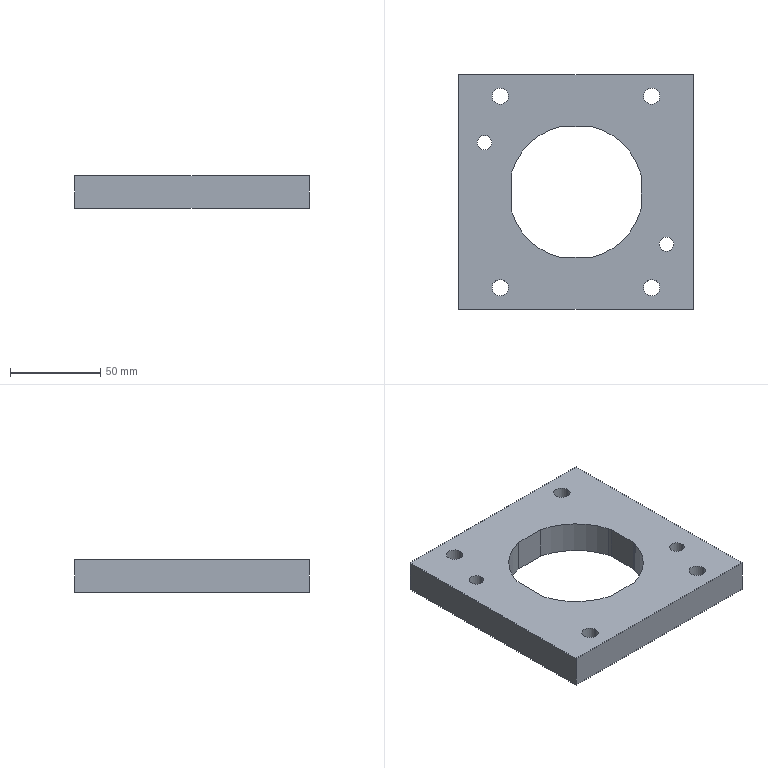Part | SolidWorks | features BaseBody 1 | 1 solid | 30 faces | box 130 x 130 x 18 mm | volume 220294 mm3 | cylinder 18 | plane 12 | commonest cylinder face diameters 9.007 x8 8 x4 74.52 x4 74.5 x2
STEP:
#1=CARTESIAN_POINT('',(-123.497,-77.99,46.3));
#2=VERTEX_POINT('',#1);
#3=CARTESIAN_POINT('',(-132.504,-77.99,46.3));
#4=VERTEX_POINT('',#3);
#5=CARTESIAN_POINT('',(-128.,-77.99,46.3));
#6=DIRECTION('',(0.,0.,-1.));
#7=DIRECTION('',(0.7071,-0.7071,0.));
#8=AXIS2_PLACEMENT_3D('',#5,#6,#7);
#9=CIRCLE('',#8,4.503);
#10=EDGE_CURVE('',#2,#4,#9,.T.);
#11=ORIENTED_EDGE('',*,*,#10,.T.);
#12=CARTESIAN_POINT('',(-132.504,-77.99,64.3));
#13=VERTEX_POINT('',#12);
#14=CARTESIAN_POINT('',(-132.504,-77.99,46.3));
#15=DIRECTION('',(0.,0.,1.));
#16=VECTOR('',#15,1000.);
#17=LINE('',#14,#16);
#18=EDGE_CURVE('',#4,#13,#17,.T.);
#19=ORIENTED_EDGE('',*,*,#18,.T.);
#20=CARTESIAN_POINT('',(-123.497,-77.99,64.3));
#21=VERTEX_POINT('',#20);
#22=CARTESIAN_POINT('',(-128.,-77.99,64.3));
#23=DIRECTION('',(0.,0.,-1.));
#24=DIRECTION('',(0.7071,-0.7071,0.));
#25=AXIS2_PLACEMENT_3D('',#22,#23,#24);
#26=CIRCLE('',#25,4.503);
#27=EDGE_CURVE('',#21,#13,#26,.T.);
#28=ORIENTED_EDGE('',*,*,#27,.F.);
#29=CARTESIAN_POINT('',(-123.497,-77.99,46.3));
#30=DIRECTION('',(0.,0.,1.));
#31=VECTOR('',#30,1000.);
#32=LINE('',#29,#31);
#33=EDGE_CURVE('',#2,#21,#32,.T.);
#34=ORIENTED_EDGE('',*,*,#33,.F.);
#35=EDGE_LOOP('',(#11,#19,#28,#34));
#36=FACE_OUTER_BOUND('',#35,.T.);
#37=CARTESIAN_POINT('',(-128.,-77.99,46.3));
#38=DIRECTION('',(0.,0.,1.));
#39=DIRECTION('',(1.,0.,0.));
#40=AXIS2_PLACEMENT_3D('',#37,#38,#39);
#41=CYLINDRICAL_SURFACE('',#40,4.503);
#42=ADVANCED_FACE('',(#36),#41,.F.);
#43=CARTESIAN_POINT('',(-48.503,27.99,46.3));
#44=VERTEX_POINT('',#43);
#45=CARTESIAN_POINT('',(-39.496,27.99,46.3));
#46=VERTEX_POINT('',#45);
#47=CARTESIAN_POINT('',(-44.,27.99,46.3));
#48=DIRECTION('',(0.,0.,-1.));
#49=DIRECTION('',(-0.7071,0.7071,0.));
#50=AXIS2_PLACEMENT_3D('',#47,#48,#49);
#51=CIRCLE('',#50,4.503);
#52=EDGE_CURVE('',#44,#46,#51,.T.);
#53=ORIENTED_EDGE('',*,*,#52,.T.);
#54=CARTESIAN_POINT('',(-39.496,27.99,64.3));
#55=VERTEX_POINT('',#54);
#56=CARTESIAN_POINT('',(-39.496,27.99,46.3));
#57=DIRECTION('',(0.,0.,1.));
#58=VECTOR('',#57,1000.);
#59=LINE('',#56,#58);
#60=EDGE_CURVE('',#46,#55,#59,.T.);
#61=ORIENTED_EDGE('',*,*,#60,.T.);
#62=CARTESIAN_POINT('',(-48.503,27.99,64.3));
#63=VERTEX_POINT('',#62);
#64=CARTESIAN_POINT('',(-44.,27.99,64.3));
#65=DIRECTION('',(0.,0.,-1.));
#66=DIRECTION('',(-0.7071,0.7071,0.));
#67=AXIS2_PLACEMENT_3D('',#64,#65,#66);
#68=CIRCLE('',#67,4.503);
#69=EDGE_CURVE('',#63,#55,#68,.T.);
#70=ORIENTED_EDGE('',*,*,#69,.F.);
#71=CARTESIAN_POINT('',(-48.503,27.99,46.3));
#72=DIRECTION('',(0.,0.,1.));
#73=VECTOR('',#72,1000.);
#74=LINE('',#71,#73);
#75=EDGE_CURVE('',#44,#63,#74,.T.);
#76=ORIENTED_EDGE('',*,*,#75,.F.);
#77=EDGE_LOOP('',(#53,#61,#70,#76));
#78=FACE_OUTER_BOUND('',#77,.T.);
#79=CARTESIAN_POINT('',(-44.,27.99,46.3));
#80=DIRECTION('',(0.,0.,1.));
#81=DIRECTION('',(-1.,0.,0.));
#82=AXIS2_PLACEMENT_3D('',#79,#80,#81);
#83=CYLINDRICAL_SURFACE('',#82,4.504);
#84=ADVANCED_FACE('',(#78),#83,.F.);
#85=CARTESIAN_POINT('',(-140.678,2.312,46.3));
#86=VERTEX_POINT('',#85);
#87=CARTESIAN_POINT('',(-132.678,2.312,46.3));
#88=VERTEX_POINT('',#87);
#89=CARTESIAN_POINT('',(-136.678,2.312,46.3));
#90=DIRECTION('',(0.,0.,1.));
#91=DIRECTION('',(0.7071,0.7071,0.));
#92=AXIS2_PLACEMENT_3D('',#89,#90,#91);
#93=CIRCLE('',#92,4.);
#94=EDGE_CURVE('',#86,#88,#93,.T.);
#95=ORIENTED_EDGE('',*,*,#94,.F.);
#96=CARTESIAN_POINT('',(-140.678,2.312,64.3));
#97=VERTEX_POINT('',#96);
#98=CARTESIAN_POINT('',(-140.678,2.312,46.3));
#99=DIRECTION('',(0.,0.,1.));
#100=VECTOR('',#99,1000.);
#101=LINE('',#98,#100);
#102=EDGE_CURVE('',#86,#97,#101,.T.);
#103=ORIENTED_EDGE('',*,*,#102,.T.);
#104=CARTESIAN_POINT('',(-132.678,2.312,64.3));
#105=VERTEX_POINT('',#104);
#106=CARTESIAN_POINT('',(-136.678,2.312,64.3));
#107=DIRECTION('',(0.,0.,1.));
#108=DIRECTION('',(0.7071,0.7071,0.));
#109=AXIS2_PLACEMENT_3D('',#106,#107,#108);
#110=CIRCLE('',#109,4.);
#111=EDGE_CURVE('',#97,#105,#110,.T.);
#112=ORIENTED_EDGE('',*,*,#111,.T.);
#113=CARTESIAN_POINT('',(-132.678,2.312,46.3));
#114=DIRECTION('',(0.,0.,1.));
#115=VECTOR('',#114,1000.);
#116=LINE('',#113,#115);
#117=EDGE_CURVE('',#88,#105,#116,.T.);
#118=ORIENTED_EDGE('',*,*,#117,.F.);
#119=EDGE_LOOP('',(#95,#103,#112,#118));
#120=FACE_OUTER_BOUND('',#119,.T.);
#121=CARTESIAN_POINT('',(-136.678,2.312,46.3));
#122=DIRECTION('',(0.,0.,1.));
#123=DIRECTION('',(1.,0.,0.));
#124=AXIS2_PLACEMENT_3D('',#121,#122,#123);
#125=CYLINDRICAL_SURFACE('',#124,4.);
#126=ADVANCED_FACE('',(#120),#125,.F.);
#127=CARTESIAN_POINT('',(-39.858,-53.934,46.3));
#128=VERTEX_POINT('',#127);
#129=CARTESIAN_POINT('',(-31.858,-53.934,46.3));
#130=VERTEX_POINT('',#129);
#131=CARTESIAN_POINT('',(-35.858,-53.934,46.3));
#132=DIRECTION('',(0.,0.,1.));
#133=DIRECTION('',(0.7071,0.7071,0.));
#134=AXIS2_PLACEMENT_3D('',#131,#132,#133);
#135=CIRCLE('',#134,4.);
#136=EDGE_CURVE('',#128,#130,#135,.T.);
#137=ORIENTED_EDGE('',*,*,#136,.F.);
#138=CARTESIAN_POINT('',(-39.858,-53.934,64.3));
#139=VERTEX_POINT('',#138);
#140=CARTESIAN_POINT('',(-39.858,-53.934,46.3));
#141=DIRECTION('',(0.,0.,1.));
#142=VECTOR('',#141,1000.);
#143=LINE('',#140,#142);
#144=EDGE_CURVE('',#128,#139,#143,.T.);
#145=ORIENTED_EDGE('',*,*,#144,.T.);
#146=CARTESIAN_POINT('',(-31.858,-53.934,64.3));
#147=VERTEX_POINT('',#146);
#148=CARTESIAN_POINT('',(-35.858,-53.934,64.3));
#149=DIRECTION('',(0.,0.,1.));
#150=DIRECTION('',(0.7071,0.7071,0.));
#151=AXIS2_PLACEMENT_3D('',#148,#149,#150);
#152=CIRCLE('',#151,4.);
#153=EDGE_CURVE('',#139,#147,#152,.T.);
#154=ORIENTED_EDGE('',*,*,#153,.T.);
#155=CARTESIAN_POINT('',(-31.858,-53.934,46.3));
#156=DIRECTION('',(0.,0.,1.));
#157=VECTOR('',#156,1000.);
#158=LINE('',#155,#157);
#159=EDGE_CURVE('',#130,#147,#158,.T.);
#160=ORIENTED_EDGE('',*,*,#159,.F.);
#161=EDGE_LOOP('',(#137,#145,#154,#160));
#162=FACE_OUTER_BOUND('',#161,.T.);
#163=CARTESIAN_POINT('',(-35.858,-53.934,46.3));
#164=DIRECTION('',(0.,0.,1.));
#165=DIRECTION('',(1.,0.,0.));
#166=AXIS2_PLACEMENT_3D('',#163,#164,#165);
#167=CYLINDRICAL_SURFACE('',#166,4.);
#168=ADVANCED_FACE('',(#162),#167,.F.);
#169=CARTESIAN_POINT('',(-39.496,-77.99,46.3));
#170=VERTEX_POINT('',#169);
#171=CARTESIAN_POINT('',(-48.503,-77.99,46.3));
#172=VERTEX_POINT('',#171);
#173=CARTESIAN_POINT('',(-44.,-77.99,46.3));
#174=DIRECTION('',(0.,0.,1.));
#175=DIRECTION('',(-0.7071,-0.7071,0.));
#176=AXIS2_PLACEMENT_3D('',#173,#174,#175);
#177=CIRCLE('',#176,4.503);
#178=EDGE_CURVE('',#170,#172,#177,.T.);
#179=ORIENTED_EDGE('',*,*,#178,.F.);
#180=CARTESIAN_POINT('',(-39.496,-77.99,64.3));
#181=VERTEX_POINT('',#180);
#182=CARTESIAN_POINT('',(-39.496,-77.99,46.3));
#183=DIRECTION('',(0.,0.,1.));
#184=VECTOR('',#183,1000.);
#185=LINE('',#182,#184);
#186=EDGE_CURVE('',#170,#181,#185,.T.);
#187=ORIENTED_EDGE('',*,*,#186,.T.);
#188=CARTESIAN_POINT('',(-48.503,-77.99,64.3));
#189=VERTEX_POINT('',#188);
#190=CARTESIAN_POINT('',(-44.,-77.99,64.3));
#191=DIRECTION('',(0.,0.,1.));
#192=DIRECTION('',(-0.7071,-0.7071,0.));
#193=AXIS2_PLACEMENT_3D('',#190,#191,#192);
#194=CIRCLE('',#193,4.503);
#195=EDGE_CURVE('',#181,#189,#194,.T.);
#196=ORIENTED_EDGE('',*,*,#195,.T.);
#197=CARTESIAN_POINT('',(-48.503,-77.99,46.3));
#198=DIRECTION('',(0.,0.,1.));
#199=VECTOR('',#198,1000.);
#200=LINE('',#197,#199);
#201=EDGE_CURVE('',#172,#189,#200,.T.);
#202=ORIENTED_EDGE('',*,*,#201,.F.);
#203=EDGE_LOOP('',(#179,#187,#196,#202));
#204=FACE_OUTER_BOUND('',#203,.T.);
#205=CARTESIAN_POINT('',(-44.,-77.99,46.3));
#206=DIRECTION('',(0.,0.,1.));
#207=DIRECTION('',(-1.,0.,0.));
#208=AXIS2_PLACEMENT_3D('',#205,#206,#207);
#209=CYLINDRICAL_SURFACE('',#208,4.504);
#210=ADVANCED_FACE('',(#204),#209,.F.);
#211=CARTESIAN_POINT('',(-132.504,27.99,46.3));
#212=VERTEX_POINT('',#211);
#213=CARTESIAN_POINT('',(-123.497,27.99,46.3));
#214=VERTEX_POINT('',#213);
#215=CARTESIAN_POINT('',(-128.,27.99,46.3));
#216=DIRECTION('',(0.,0.,1.));
#217=DIRECTION('',(0.7071,0.7071,0.));
#218=AXIS2_PLACEMENT_3D('',#215,#216,#217);
#219=CIRCLE('',#218,4.504);
#220=EDGE_CURVE('',#212,#214,#219,.T.);
#221=ORIENTED_EDGE('',*,*,#220,.F.);
#222=CARTESIAN_POINT('',(-132.504,27.99,64.3));
#223=VERTEX_POINT('',#222);
#224=CARTESIAN_POINT('',(-132.504,27.99,46.3));
#225=DIRECTION('',(0.,0.,1.));
#226=VECTOR('',#225,1000.);
#227=LINE('',#224,#226);
#228=EDGE_CURVE('',#212,#223,#227,.T.);
#229=ORIENTED_EDGE('',*,*,#228,.T.);
#230=CARTESIAN_POINT('',(-123.497,27.99,64.3));
#231=VERTEX_POINT('',#230);
#232=CARTESIAN_POINT('',(-128.,27.99,64.3));
#233=DIRECTION('',(0.,0.,1.));
#234=DIRECTION('',(0.7071,0.7071,0.));
#235=AXIS2_PLACEMENT_3D('',#232,#233,#234);
#236=CIRCLE('',#235,4.504);
#237=EDGE_CURVE('',#223,#231,#236,.T.);
#238=ORIENTED_EDGE('',*,*,#237,.T.);
#239=CARTESIAN_POINT('',(-123.497,27.99,46.3));
#240=DIRECTION('',(0.,0.,1.));
#241=VECTOR('',#240,1000.);
#242=LINE('',#239,#241);
#243=EDGE_CURVE('',#214,#231,#242,.T.);
#244=ORIENTED_EDGE('',*,*,#243,.F.);
#245=EDGE_LOOP('',(#221,#229,#238,#244));
#246=FACE_OUTER_BOUND('',#245,.T.);
#247=CARTESIAN_POINT('',(-128.,27.99,46.3));
#248=DIRECTION('',(0.,0.,1.));
#249=DIRECTION('',(1.,0.,0.));
#250=AXIS2_PLACEMENT_3D('',#247,#248,#249);
#251=CYLINDRICAL_SURFACE('',#250,4.503);
#252=ADVANCED_FACE('',(#246),#251,.F.);
#253=CARTESIAN_POINT('',(-50.24,-14.57,64.3));
#254=VERTEX_POINT('',#253);
#255=CARTESIAN_POINT('',(-50.24,-14.57,46.3));
#256=VERTEX_POINT('',#255);
#257=CARTESIAN_POINT('',(-50.24,-14.57,46.3));
#258=DIRECTION('',(0.,0.,-1.));
#259=VECTOR('',#258,1000.);
#260=LINE('',#257,#259);
#261=EDGE_CURVE('',#254,#256,#260,.T.);
#262=ORIENTED_EDGE('',*,*,#261,.F.);
#263=CARTESIAN_POINT('',(-50.24,-14.534,64.3));
#264=VERTEX_POINT('',#263);
#265=CARTESIAN_POINT('',(-50.24,-25.,64.3));
#266=DIRECTION('',(0.,1.,0.));
#267=VECTOR('',#266,1000.);
#268=LINE('',#265,#267);
#269=EDGE_CURVE('',#254,#264,#268,.T.);
#270=ORIENTED_EDGE('',*,*,#269,.T.);
#271=CARTESIAN_POINT('',(-50.24,-14.534,46.3));
#272=VERTEX_POINT('',#271);
#273=CARTESIAN_POINT('',(-50.24,-14.534,64.3));
#274=DIRECTION('',(0.,0.,-1.));
#275=VECTOR('',#274,1000.);
#276=LINE('',#273,#275);
#277=EDGE_CURVE('',#264,#272,#276,.T.);
#278=ORIENTED_EDGE('',*,*,#277,.T.);
#279=CARTESIAN_POINT('',(-50.24,-25.,46.3));
#280=DIRECTION('',(0.,1.,0.));
#281=VECTOR('',#280,1000.);
#282=LINE('',#279,#281);
#283=EDGE_CURVE('',#256,#272,#282,.T.);
#284=ORIENTED_EDGE('',*,*,#283,.F.);
#285=EDGE_LOOP('',(#262,#270,#278,#284));
#286=FACE_OUTER_BOUND('',#285,.T.);
#287=CARTESIAN_POINT('',(-50.24,-25.,46.3));
#288=DIRECTION('',(1.,0.,0.));
#289=DIRECTION('',(0.,1.,0.));
#290=AXIS2_PLACEMENT_3D('',#287,#288,#289);
#291=PLANE('',#290);
#292=ADVANCED_FACE('',(#286),#291,.F.);
#293=ORIENTED_EDGE('',*,*,#27,.T.);
#294=CARTESIAN_POINT('',(-128.,-77.99,64.3));
#295=DIRECTION('',(0.,0.,-1.));
#296=DIRECTION('',(0.7071,-0.7071,0.));
#297=AXIS2_PLACEMENT_3D('',#294,#295,#296);
#298=CIRCLE('',#297,4.503);
#299=EDGE_CURVE('',#13,#21,#298,.T.);
#300=ORIENTED_EDGE('',*,*,#299,.T.);
#301=EDGE_LOOP('',(#293,#300));
#302=FACE_BOUND('',#301,.T.);
#303=ORIENTED_EDGE('',*,*,#69,.T.);
#304=CARTESIAN_POINT('',(-44.,27.99,64.3));
#305=DIRECTION('',(0.,0.,-1.));
#306=DIRECTION('',(-0.7071,0.7071,0.));
#307=AXIS2_PLACEMENT_3D('',#304,#305,#306);
#308=CIRCLE('',#307,4.503);
#309=EDGE_CURVE('',#55,#63,#308,.T.);
#310=ORIENTED_EDGE('',*,*,#309,.T.);
#311=EDGE_LOOP('',(#303,#310));
#312=FACE_BOUND('',#311,.T.);
#313=CARTESIAN_POINT('',(-136.678,2.312,64.3));
#314=DIRECTION('',(0.,0.,1.));
#315=DIRECTION('',(0.7071,0.7071,0.));
#316=AXIS2_PLACEMENT_3D('',#313,#314,#315);
#317=CIRCLE('',#316,4.);
#318=EDGE_CURVE('',#105,#97,#317,.T.);
#319=ORIENTED_EDGE('',*,*,#318,.F.);
#320=ORIENTED_EDGE('',*,*,#111,.F.);
#321=EDGE_LOOP('',(#319,#320));
#322=FACE_BOUND('',#321,.T.);
#323=CARTESIAN_POINT('',(-35.858,-53.934,64.3));
#324=DIRECTION('',(0.,0.,1.));
#325=DIRECTION('',(0.7071,0.7071,0.));
#326=AXIS2_PLACEMENT_3D('',#323,#324,#325);
#327=CIRCLE('',#326,4.);
#328=EDGE_CURVE('',#147,#139,#327,.T.);
#329=ORIENTED_EDGE('',*,*,#328,.F.);
#330=ORIENTED_EDGE('',*,*,#153,.F.);
#331=EDGE_LOOP('',(#329,#330));
#332=FACE_BOUND('',#331,.T.);
#333=CARTESIAN_POINT('',(-44.,-77.99,64.3));
#334=DIRECTION('',(0.,0.,1.));
#335=DIRECTION('',(-0.7071,-0.7071,0.));
#336=AXIS2_PLACEMENT_3D('',#333,#334,#335);
#337=CIRCLE('',#336,4.503);
#338=EDGE_CURVE('',#189,#181,#337,.T.);
#339=ORIENTED_EDGE('',*,*,#338,.F.);
#340=ORIENTED_EDGE('',*,*,#195,.F.);
#341=EDGE_LOOP('',(#339,#340));
#342=FACE_BOUND('',#341,.T.);
#343=CARTESIAN_POINT('',(-128.,27.99,64.3));
#344=DIRECTION('',(0.,0.,1.));
#345=DIRECTION('',(0.7071,0.7071,0.));
#346=AXIS2_PLACEMENT_3D('',#343,#344,#345);
#347=CIRCLE('',#346,4.504);
#348=EDGE_CURVE('',#231,#223,#347,.T.);
#349=ORIENTED_EDGE('',*,*,#348,.F.);
#350=ORIENTED_EDGE('',*,*,#237,.F.);
#351=EDGE_LOOP('',(#349,#350));
#352=FACE_BOUND('',#351,.T.);
#353=CARTESIAN_POINT('',(-151.,-90.,64.3));
#354=VERTEX_POINT('',#353);
#355=CARTESIAN_POINT('',(-21.,-90.,64.3));
#356=VERTEX_POINT('',#355);
#357=CARTESIAN_POINT('',(-86.,-90.,64.3));
#358=DIRECTION('',(1.,0.,0.));
#359=VECTOR('',#358,1000.);
#360=LINE('',#357,#359);
#361=EDGE_CURVE('',#354,#356,#360,.T.);
#362=ORIENTED_EDGE('',*,*,#361,.T.);
#363=CARTESIAN_POINT('',(-21.,40.,64.3));
#364=VERTEX_POINT('',#363);
#365=CARTESIAN_POINT('',(-21.,-25.,64.3));
#366=DIRECTION('',(0.,1.,0.));
#367=VECTOR('',#366,1000.);
#368=LINE('',#365,#367);
#369=EDGE_CURVE('',#356,#364,#368,.T.);
#370=ORIENTED_EDGE('',*,*,#369,.T.);
#371=CARTESIAN_POINT('',(-151.,40.,64.3));
#372=VERTEX_POINT('',#371);
#373=CARTESIAN_POINT('',(-86.,40.,64.3));
#374=DIRECTION('',(-1.,0.,0.));
#375=VECTOR('',#374,1000.);
#376=LINE('',#373,#375);
#377=EDGE_CURVE('',#364,#372,#376,.T.);
#378=ORIENTED_EDGE('',*,*,#377,.T.);
#379=CARTESIAN_POINT('',(-151.,-25.,64.3));
#380=DIRECTION('',(0.,-1.,0.));
#381=VECTOR('',#380,1000.);
#382=LINE('',#379,#381);
#383=EDGE_CURVE('',#372,#354,#382,.T.);
#384=ORIENTED_EDGE('',*,*,#383,.T.);
#385=EDGE_LOOP('',(#362,#370,#378,#384));
#386=FACE_OUTER_BOUND('',#385,.T.);
#387=CARTESIAN_POINT('',(-49.74,-33.531,64.3));
#388=VERTEX_POINT('',#387);
#389=CARTESIAN_POINT('',(-49.74,-16.469,64.3));
#390=VERTEX_POINT('',#389);
#391=CARTESIAN_POINT('',(-49.74,-25.,64.3));
#392=DIRECTION('',(0.,1.,0.));
#393=VECTOR('',#392,1000.);
#394=LINE('',#391,#393);
#395=EDGE_CURVE('',#388,#390,#394,.T.);
#396=ORIENTED_EDGE('',*,*,#395,.F.);
#397=CARTESIAN_POINT('',(-50.24,-35.43,64.3));
#398=VERTEX_POINT('',#397);
#399=CARTESIAN_POINT('',(-86.,-25.,64.3));
#400=DIRECTION('',(0.,0.,-1.));
#401=DIRECTION('',(-1.,0.,0.));
#402=AXIS2_PLACEMENT_3D('',#399,#400,#401);
#403=CIRCLE('',#402,37.25);
#404=EDGE_CURVE('',#388,#398,#403,.T.);
#405=ORIENTED_EDGE('',*,*,#404,.T.);
#406=CARTESIAN_POINT('',(-50.24,-35.466,64.3));
#407=VERTEX_POINT('',#406);
#408=CARTESIAN_POINT('',(-50.24,-25.,64.3));
#409=DIRECTION('',(0.,1.,0.));
#410=VECTOR('',#409,1000.);
#411=LINE('',#408,#410);
#412=EDGE_CURVE('',#407,#398,#411,.T.);
#413=ORIENTED_EDGE('',*,*,#412,.F.);
#414=CARTESIAN_POINT('',(-77.426,-61.26,64.3));
#415=VERTEX_POINT('',#414);
#416=CARTESIAN_POINT('',(-86.,-25.,64.3));
#417=DIRECTION('',(0.,0.,-1.));
#418=DIRECTION('',(-1.,0.,0.));
#419=AXIS2_PLACEMENT_3D('',#416,#417,#418);
#420=CIRCLE('',#419,37.26);
#421=EDGE_CURVE('',#407,#415,#420,.T.);
#422=ORIENTED_EDGE('',*,*,#421,.T.);
#423=CARTESIAN_POINT('',(-94.574,-61.26,64.3));
#424=VERTEX_POINT('',#423);
#425=CARTESIAN_POINT('',(-86.,-61.26,64.3));
#426=DIRECTION('',(-1.,0.,0.));
#427=VECTOR('',#426,1000.);
#428=LINE('',#425,#427);
#429=EDGE_CURVE('',#415,#424,#428,.T.);
#430=ORIENTED_EDGE('',*,*,#429,.T.);
#431=CARTESIAN_POINT('',(-121.76,-35.466,64.3));
#432=VERTEX_POINT('',#431);
#433=CARTESIAN_POINT('',(-86.,-25.,64.3));
#434=DIRECTION('',(0.,0.,-1.));
#435=DIRECTION('',(-1.,0.,0.));
#436=AXIS2_PLACEMENT_3D('',#433,#434,#435);
#437=CIRCLE('',#436,37.26);
#438=EDGE_CURVE('',#424,#432,#437,.T.);
#439=ORIENTED_EDGE('',*,*,#438,.T.);
#440=CARTESIAN_POINT('',(-121.76,-14.534,64.3));
#441=VERTEX_POINT('',#440);
#442=CARTESIAN_POINT('',(-121.76,-25.,64.3));
#443=DIRECTION('',(0.,1.,0.));
#444=VECTOR('',#443,1000.);
#445=LINE('',#442,#444);
#446=EDGE_CURVE('',#432,#441,#445,.T.);
#447=ORIENTED_EDGE('',*,*,#446,.T.);
#448=CARTESIAN_POINT('',(-94.574,11.26,64.3));
#449=VERTEX_POINT('',#448);
#450=CARTESIAN_POINT('',(-86.,-25.,64.3));
#451=DIRECTION('',(0.,0.,-1.));
#452=DIRECTION('',(-1.,0.,0.));
#453=AXIS2_PLACEMENT_3D('',#450,#451,#452);
#454=CIRCLE('',#453,37.26);
#455=EDGE_CURVE('',#441,#449,#454,.T.);
#456=ORIENTED_EDGE('',*,*,#455,.T.);
#457=CARTESIAN_POINT('',(-77.426,11.26,64.3));
#458=VERTEX_POINT('',#457);
#459=CARTESIAN_POINT('',(-86.,11.26,64.3));
#460=DIRECTION('',(1.,0.,0.));
#461=VECTOR('',#460,1000.);
#462=LINE('',#459,#461);
#463=EDGE_CURVE('',#449,#458,#462,.T.);
#464=ORIENTED_EDGE('',*,*,#463,.T.);
#465=CARTESIAN_POINT('',(-86.,-25.,64.3));
#466=DIRECTION('',(0.,0.,-1.));
#467=DIRECTION('',(-1.,0.,0.));
#468=AXIS2_PLACEMENT_3D('',#465,#466,#467);
#469=CIRCLE('',#468,37.26);
#470=EDGE_CURVE('',#458,#264,#469,.T.);
#471=ORIENTED_EDGE('',*,*,#470,.T.);
#472=ORIENTED_EDGE('',*,*,#269,.F.);
#473=CARTESIAN_POINT('',(-86.,-25.,64.3));
#474=DIRECTION('',(0.,0.,-1.));
#475=DIRECTION('',(-1.,0.,0.));
#476=AXIS2_PLACEMENT_3D('',#473,#474,#475);
#477=CIRCLE('',#476,37.25);
#478=EDGE_CURVE('',#254,#390,#477,.T.);
#479=ORIENTED_EDGE('',*,*,#478,.T.);
#480=EDGE_LOOP('',(#396,#405,#413,#422,#430,#439,#447,#456,#464,#471,#472,#479));
#481=FACE_BOUND('',#480,.T.);
#482=CARTESIAN_POINT('',(-86.,-25.,64.3));
#483=DIRECTION('',(0.,0.,-1.));
#484=DIRECTION('',(-1.,0.,0.));
#485=AXIS2_PLACEMENT_3D('',#482,#483,#484);
#486=PLANE('',#485);
#487=ADVANCED_FACE('',(#302,#312,#322,#332,#342,#352,#386,#481),#486,.F.);
#488=CARTESIAN_POINT('',(-49.74,-16.469,46.3));
#489=VERTEX_POINT('',#488);
#490=CARTESIAN_POINT('',(-86.,-25.,46.3));
#491=DIRECTION('',(0.,0.,-1.));
#492=DIRECTION('',(-1.,0.,0.));
#493=AXIS2_PLACEMENT_3D('',#490,#491,#492);
#494=CIRCLE('',#493,37.25);
#495=EDGE_CURVE('',#256,#489,#494,.T.);
#496=ORIENTED_EDGE('',*,*,#495,.F.);
#497=ORIENTED_EDGE('',*,*,#283,.T.);
#498=CARTESIAN_POINT('',(-77.426,11.26,46.3));
#499=VERTEX_POINT('',#498);
#500=CARTESIAN_POINT('',(-86.,-25.,46.3));
#501=DIRECTION('',(0.,0.,-1.));
#502=DIRECTION('',(-1.,0.,0.));
#503=AXIS2_PLACEMENT_3D('',#500,#501,#502);
#504=CIRCLE('',#503,37.26);
#505=EDGE_CURVE('',#499,#272,#504,.T.);
#506=ORIENTED_EDGE('',*,*,#505,.F.);
#507=CARTESIAN_POINT('',(-94.574,11.26,46.3));
#508=VERTEX_POINT('',#507);
#509=CARTESIAN_POINT('',(-86.,11.26,46.3));
#510=DIRECTION('',(1.,0.,0.));
#511=VECTOR('',#510,1000.);
#512=LINE('',#509,#511);
#513=EDGE_CURVE('',#508,#499,#512,.T.);
#514=ORIENTED_EDGE('',*,*,#513,.F.);
#515=CARTESIAN_POINT('',(-121.76,-14.534,46.3));
#516=VERTEX_POINT('',#515);
#517=CARTESIAN_POINT('',(-86.,-25.,46.3));
#518=DIRECTION('',(0.,0.,-1.));
#519=DIRECTION('',(-1.,0.,0.));
#520=AXIS2_PLACEMENT_3D('',#517,#518,#519);
#521=CIRCLE('',#520,37.26);
#522=EDGE_CURVE('',#516,#508,#521,.T.);
#523=ORIENTED_EDGE('',*,*,#522,.F.);
#524=CARTESIAN_POINT('',(-121.76,-35.466,46.3));
#525=VERTEX_POINT('',#524);
#526=CARTESIAN_POINT('',(-121.76,-25.,46.3));
#527=DIRECTION('',(0.,1.,0.));
#528=VECTOR('',#527,1000.);
#529=LINE('',#526,#528);
#530=EDGE_CURVE('',#525,#516,#529,.T.);
#531=ORIENTED_EDGE('',*,*,#530,.F.);
#532=CARTESIAN_POINT('',(-94.574,-61.26,46.3));
#533=VERTEX_POINT('',#532);
#534=CARTESIAN_POINT('',(-86.,-25.,46.3));
#535=DIRECTION('',(0.,0.,-1.));
#536=DIRECTION('',(-1.,0.,0.));
#537=AXIS2_PLACEMENT_3D('',#534,#535,#536);
#538=CIRCLE('',#537,37.26);
#539=EDGE_CURVE('',#533,#525,#538,.T.);
#540=ORIENTED_EDGE('',*,*,#539,.F.);
#541=CARTESIAN_POINT('',(-77.426,-61.26,46.3));
#542=VERTEX_POINT('',#541);
#543=CARTESIAN_POINT('',(-86.,-61.26,46.3));
#544=DIRECTION('',(1.,0.,0.));
#545=VECTOR('',#544,1000.);
#546=LINE('',#543,#545);
#547=EDGE_CURVE('',#533,#542,#546,.T.);
#548=ORIENTED_EDGE('',*,*,#547,.T.);
#549=CARTESIAN_POINT('',(-50.24,-35.466,46.3));
#550=VERTEX_POINT('',#549);
#551=CARTESIAN_POINT('',(-86.,-25.,46.3));
#552=DIRECTION('',(0.,0.,-1.));
#553=DIRECTION('',(-1.,0.,0.));
#554=AXIS2_PLACEMENT_3D('',#551,#552,#553);
#555=CIRCLE('',#554,37.26);
#556=EDGE_CURVE('',#550,#542,#555,.T.);
#557=ORIENTED_EDGE('',*,*,#556,.F.);
#558=CARTESIAN_POINT('',(-50.24,-35.43,46.3));
#559=VERTEX_POINT('',#558);
#560=CARTESIAN_POINT('',(-50.24,-25.,46.3));
#561=DIRECTION('',(0.,1.,0.));
#562=VECTOR('',#561,1000.);
#563=LINE('',#560,#562);
#564=EDGE_CURVE('',#550,#559,#563,.T.);
#565=ORIENTED_EDGE('',*,*,#564,.T.);
#566=CARTESIAN_POINT('',(-49.74,-33.531,46.3));
#567=VERTEX_POINT('',#566);
#568=CARTESIAN_POINT('',(-86.,-25.,46.3));
#569=DIRECTION('',(0.,0.,-1.));
#570=DIRECTION('',(-1.,0.,0.));
#571=AXIS2_PLACEMENT_3D('',#568,#569,#570);
#572=CIRCLE('',#571,37.25);
#573=EDGE_CURVE('',#567,#559,#572,.T.);
#574=ORIENTED_EDGE('',*,*,#573,.F.);
#575=CARTESIAN_POINT('',(-49.74,-25.,46.3));
#576=DIRECTION('',(0.,1.,0.));
#577=VECTOR('',#576,1000.);
#578=LINE('',#575,#577);
#579=EDGE_CURVE('',#567,#489,#578,.T.);
#580=ORIENTED_EDGE('',*,*,#579,.T.);
#581=EDGE_LOOP('',(#496,#497,#506,#514,#523,#531,#540,#548,#557,#565,#574,#580));
#582=FACE_BOUND('',#581,.T.);
#583=ORIENTED_EDGE('',*,*,#10,.F.);
#584=CARTESIAN_POINT('',(-128.,-77.99,46.3));
#585=DIRECTION('',(0.,0.,-1.));
#586=DIRECTION('',(0.7071,-0.7071,0.));
#587=AXIS2_PLACEMENT_3D('',#584,#585,#586);
#588=CIRCLE('',#587,4.503);
#589=EDGE_CURVE('',#4,#2,#588,.T.);
#590=ORIENTED_EDGE('',*,*,#589,.F.);
#591=EDGE_LOOP('',(#583,#590));
#592=FACE_BOUND('',#591,.T.);
#593=ORIENTED_EDGE('',*,*,#52,.F.);
#594=CARTESIAN_POINT('',(-44.,27.99,46.3));
#595=DIRECTION('',(0.,0.,-1.));
#596=DIRECTION('',(-0.7071,0.7071,0.));
#597=AXIS2_PLACEMENT_3D('',#594,#595,#596);
#598=CIRCLE('',#597,4.503);
#599=EDGE_CURVE('',#46,#44,#598,.T.);
#600=ORIENTED_EDGE('',*,*,#599,.F.);
#601=EDGE_LOOP('',(#593,#600));
#602=FACE_BOUND('',#601,.T.);
#603=CARTESIAN_POINT('',(-136.678,2.312,46.3));
#604=DIRECTION('',(0.,0.,1.));
#605=DIRECTION('',(0.7071,0.7071,0.));
#606=AXIS2_PLACEMENT_3D('',#603,#604,#605);
#607=CIRCLE('',#606,4.);
#608=EDGE_CURVE('',#88,#86,#607,.T.);
#609=ORIENTED_EDGE('',*,*,#608,.T.);
#610=ORIENTED_EDGE('',*,*,#94,.T.);
#611=EDGE_LOOP('',(#609,#610));
#612=FACE_BOUND('',#611,.T.);
#613=CARTESIAN_POINT('',(-35.858,-53.934,46.3));
#614=DIRECTION('',(0.,0.,1.));
#615=DIRECTION('',(0.7071,0.7071,0.));
#616=AXIS2_PLACEMENT_3D('',#613,#614,#615);
#617=CIRCLE('',#616,4.);
#618=EDGE_CURVE('',#130,#128,#617,.T.);
#619=ORIENTED_EDGE('',*,*,#618,.T.);
#620=ORIENTED_EDGE('',*,*,#136,.T.);
#621=EDGE_LOOP('',(#619,#620));
#622=FACE_BOUND('',#621,.T.);
#623=CARTESIAN_POINT('',(-44.,-77.99,46.3));
#624=DIRECTION('',(0.,0.,1.));
#625=DIRECTION('',(-0.7071,-0.7071,0.));
#626=AXIS2_PLACEMENT_3D('',#623,#624,#625);
#627=CIRCLE('',#626,4.503);
#628=EDGE_CURVE('',#172,#170,#627,.T.);
#629=ORIENTED_EDGE('',*,*,#628,.T.);
#630=ORIENTED_EDGE('',*,*,#178,.T.);
#631=EDGE_LOOP('',(#629,#630));
#632=FACE_BOUND('',#631,.T.);
#633=CARTESIAN_POINT('',(-128.,27.99,46.3));
#634=DIRECTION('',(0.,0.,1.));
#635=DIRECTION('',(0.7071,0.7071,0.));
#636=AXIS2_PLACEMENT_3D('',#633,#634,#635);
#637=CIRCLE('',#636,4.504);
#638=EDGE_CURVE('',#214,#212,#637,.T.);
#639=ORIENTED_EDGE('',*,*,#638,.T.);
#640=ORIENTED_EDGE('',*,*,#220,.T.);
#641=EDGE_LOOP('',(#639,#640));
#642=FACE_BOUND('',#641,.T.);
#643=CARTESIAN_POINT('',(-151.,-90.,46.3));
#644=VERTEX_POINT('',#643);
#645=CARTESIAN_POINT('',(-21.,-90.,46.3));
#646=VERTEX_POINT('',#645);
#647=CARTESIAN_POINT('',(-86.,-90.,46.3));
#648=DIRECTION('',(1.,0.,0.));
#649=VECTOR('',#648,1000.);
#650=LINE('',#647,#649);
#651=EDGE_CURVE('',#644,#646,#650,.T.);
#652=ORIENTED_EDGE('',*,*,#651,.F.);
#653=CARTESIAN_POINT('',(-151.,40.,46.3));
#654=VERTEX_POINT('',#653);
#655=CARTESIAN_POINT('',(-151.,-25.,46.3));
#656=DIRECTION('',(0.,-1.,0.));
#657=VECTOR('',#656,1000.);
#658=LINE('',#655,#657);
#659=EDGE_CURVE('',#654,#644,#658,.T.);
#660=ORIENTED_EDGE('',*,*,#659,.F.);
#661=CARTESIAN_POINT('',(-21.,40.,46.3));
#662=VERTEX_POINT('',#661);
#663=CARTESIAN_POINT('',(-86.,40.,46.3));
#664=DIRECTION('',(-1.,0.,0.));
#665=VECTOR('',#664,1000.);
#666=LINE('',#663,#665);
#667=EDGE_CURVE('',#662,#654,#666,.T.);
#668=ORIENTED_EDGE('',*,*,#667,.F.);
#669=CARTESIAN_POINT('',(-21.,-25.,46.3));
#670=DIRECTION('',(0.,1.,0.));
#671=VECTOR('',#670,1000.);
#672=LINE('',#669,#671);
#673=EDGE_CURVE('',#646,#662,#672,.T.);
#674=ORIENTED_EDGE('',*,*,#673,.F.);
#675=EDGE_LOOP('',(#652,#660,#668,#674));
#676=FACE_OUTER_BOUND('',#675,.T.);
#677=CARTESIAN_POINT('',(-86.,-25.,46.3));
#678=DIRECTION('',(0.,0.,-1.));
#679=DIRECTION('',(-1.,0.,0.));
#680=AXIS2_PLACEMENT_3D('',#677,#678,#679);
#681=PLANE('',#680);
#682=ADVANCED_FACE('',(#582,#592,#602,#612,#622,#632,#642,#676),#681,.T.);
#683=CARTESIAN_POINT('',(-21.,40.,46.3));
#684=DIRECTION('',(0.,0.,1.));
#685=VECTOR('',#684,1000.);
#686=LINE('',#683,#685);
#687=EDGE_CURVE('',#662,#364,#686,.T.);
#688=ORIENTED_EDGE('',*,*,#687,.F.);
#689=ORIENTED_EDGE('',*,*,#667,.T.);
#690=CARTESIAN_POINT('',(-151.,40.,46.3));
#691=DIRECTION('',(0.,0.,1.));
#692=VECTOR('',#691,1000.);
#693=LINE('',#690,#692);
#694=EDGE_CURVE('',#654,#372,#693,.T.);
#695=ORIENTED_EDGE('',*,*,#694,.T.);
#696=ORIENTED_EDGE('',*,*,#377,.F.);
#697=EDGE_LOOP('',(#688,#689,#695,#696));
#698=FACE_OUTER_BOUND('',#697,.T.);
#699=CARTESIAN_POINT('',(-86.,40.,46.3));
#700=DIRECTION('',(0.,-1.,0.));
#701=DIRECTION('',(-1.,0.,0.));
#702=AXIS2_PLACEMENT_3D('',#699,#700,#701);
#703=PLANE('',#702);
#704=ADVANCED_FACE('',(#698),#703,.F.);
#705=ORIENTED_EDGE('',*,*,#694,.F.);
#706=ORIENTED_EDGE('',*,*,#659,.T.);
#707=CARTESIAN_POINT('',(-151.,-90.,46.3));
#708=DIRECTION('',(0.,0.,1.));
#709=VECTOR('',#708,1000.);
#710=LINE('',#707,#709);
#711=EDGE_CURVE('',#644,#354,#710,.T.);
#712=ORIENTED_EDGE('',*,*,#711,.T.);
#713=ORIENTED_EDGE('',*,*,#383,.F.);
#714=EDGE_LOOP('',(#705,#706,#712,#713));
#715=FACE_OUTER_BOUND('',#714,.T.);
#716=CARTESIAN_POINT('',(-151.,-25.,46.3));
#717=DIRECTION('',(-1.,0.,0.));
#718=DIRECTION('',(0.,1.,0.));
#719=AXIS2_PLACEMENT_3D('',#716,#717,#718);
#720=PLANE('',#719);
#721=ADVANCED_FACE('',(#715),#720,.T.);
#722=ORIENTED_EDGE('',*,*,#711,.F.);
#723=ORIENTED_EDGE('',*,*,#651,.T.);
#724=CARTESIAN_POINT('',(-21.,-90.,46.3));
#725=DIRECTION('',(0.,0.,1.));
#726=VECTOR('',#725,1000.);
#727=LINE('',#724,#726);
#728=EDGE_CURVE('',#646,#356,#727,.T.);
#729=ORIENTED_EDGE('',*,*,#728,.T.);
#730=ORIENTED_EDGE('',*,*,#361,.F.);
#731=EDGE_LOOP('',(#722,#723,#729,#730));
#732=FACE_OUTER_BOUND('',#731,.T.);
#733=CARTESIAN_POINT('',(-86.,-90.,46.3));
#734=DIRECTION('',(0.,-1.,0.));
#735=DIRECTION('',(-1.,0.,0.));
#736=AXIS2_PLACEMENT_3D('',#733,#734,#735);
#737=PLANE('',#736);
#738=ADVANCED_FACE('',(#732),#737,.T.);
#739=ORIENTED_EDGE('',*,*,#673,.T.);
#740=ORIENTED_EDGE('',*,*,#687,.T.);
#741=ORIENTED_EDGE('',*,*,#369,.F.);
#742=ORIENTED_EDGE('',*,*,#728,.F.);
#743=EDGE_LOOP('',(#739,#740,#741,#742));
#744=FACE_OUTER_BOUND('',#743,.T.);
#745=CARTESIAN_POINT('',(-21.,-25.,46.3));
#746=DIRECTION('',(-1.,0.,0.));
#747=DIRECTION('',(0.,1.,0.));
#748=AXIS2_PLACEMENT_3D('',#745,#746,#747);
#749=PLANE('',#748);
#750=ADVANCED_FACE('',(#744),#749,.F.);
#751=CARTESIAN_POINT('',(-50.24,-35.43,46.3));
#752=DIRECTION('',(0.,0.,1.));
#753=VECTOR('',#752,1000.);
#754=LINE('',#751,#753);
#755=EDGE_CURVE('',#559,#398,#754,.T.);
#756=ORIENTED_EDGE('',*,*,#755,.F.);
#757=ORIENTED_EDGE('',*,*,#564,.F.);
#758=CARTESIAN_POINT('',(-50.24,-35.466,46.3));
#759=DIRECTION('',(0.,0.,1.));
#760=VECTOR('',#759,1000.);
#761=LINE('',#758,#760);
#762=EDGE_CURVE('',#550,#407,#761,.T.);
#763=ORIENTED_EDGE('',*,*,#762,.T.);
#764=ORIENTED_EDGE('',*,*,#412,.T.);
#765=EDGE_LOOP('',(#756,#757,#763,#764));
#766=FACE_OUTER_BOUND('',#765,.T.);
#767=CARTESIAN_POINT('',(-50.24,-25.,46.3));
#768=DIRECTION('',(1.,0.,0.));
#769=DIRECTION('',(0.,1.,0.));
#770=AXIS2_PLACEMENT_3D('',#767,#768,#769);
#771=PLANE('',#770);
#772=ADVANCED_FACE('',(#766),#771,.F.);
#773=ORIENTED_EDGE('',*,*,#530,.T.);
#774=CARTESIAN_POINT('',(-121.76,-14.534,46.3));
#775=DIRECTION('',(0.,0.,1.));
#776=VECTOR('',#775,1000.);
#777=LINE('',#774,#776);
#778=EDGE_CURVE('',#516,#441,#777,.T.);
#779=ORIENTED_EDGE('',*,*,#778,.T.);
#780=ORIENTED_EDGE('',*,*,#446,.F.);
#781=CARTESIAN_POINT('',(-121.76,-35.466,64.3));
#782=DIRECTION('',(0.,0.,-1.));
#783=VECTOR('',#782,1000.);
#784=LINE('',#781,#783);
#785=EDGE_CURVE('',#432,#525,#784,.T.);
#786=ORIENTED_EDGE('',*,*,#785,.T.);
#787=EDGE_LOOP('',(#773,#779,#780,#786));
#788=FACE_OUTER_BOUND('',#787,.T.);
#789=CARTESIAN_POINT('',(-121.76,-25.,46.3));
#790=DIRECTION('',(-1.,0.,0.));
#791=DIRECTION('',(0.,1.,0.));
#792=AXIS2_PLACEMENT_3D('',#789,#790,#791);
#793=PLANE('',#792);
#794=ADVANCED_FACE('',(#788),#793,.F.);
#795=CARTESIAN_POINT('',(-77.426,11.26,46.3));
#796=DIRECTION('',(0.,0.,1.));
#797=VECTOR('',#796,1000.);
#798=LINE('',#795,#797);
#799=EDGE_CURVE('',#499,#458,#798,.T.);
#800=ORIENTED_EDGE('',*,*,#799,.F.);
#801=ORIENTED_EDGE('',*,*,#505,.T.);
#802=ORIENTED_EDGE('',*,*,#277,.F.);
#803=ORIENTED_EDGE('',*,*,#470,.F.);
#804=EDGE_LOOP('',(#800,#801,#802,#803));
#805=FACE_OUTER_BOUND('',#804,.T.);
#806=CARTESIAN_POINT('',(-86.,-25.,46.3));
#807=DIRECTION('',(0.,0.,-1.));
#808=DIRECTION('',(-1.,0.,0.));
#809=AXIS2_PLACEMENT_3D('',#806,#807,#808);
#810=CYLINDRICAL_SURFACE('',#809,37.26);
#811=ADVANCED_FACE('',(#805),#810,.F.);
#812=CARTESIAN_POINT('',(-94.574,-61.26,46.3));
#813=DIRECTION('',(0.,0.,1.));
#814=VECTOR('',#813,1000.);
#815=LINE('',#812,#814);
#816=EDGE_CURVE('',#533,#424,#815,.T.);
#817=ORIENTED_EDGE('',*,*,#816,.F.);
#818=ORIENTED_EDGE('',*,*,#539,.T.);
#819=ORIENTED_EDGE('',*,*,#785,.F.);
#820=ORIENTED_EDGE('',*,*,#438,.F.);
#821=EDGE_LOOP('',(#817,#818,#819,#820));
#822=FACE_OUTER_BOUND('',#821,.T.);
#823=CARTESIAN_POINT('',(-86.,-25.,46.3));
#824=DIRECTION('',(0.,0.,-1.));
#825=DIRECTION('',(-1.,0.,0.));
#826=AXIS2_PLACEMENT_3D('',#823,#824,#825);
#827=CYLINDRICAL_SURFACE('',#826,37.26);
#828=ADVANCED_FACE('',(#822),#827,.F.);
#829=CARTESIAN_POINT('',(-94.574,11.26,64.3));
#830=DIRECTION('',(0.,0.,-1.));
#831=VECTOR('',#830,1000.);
#832=LINE('',#829,#831);
#833=EDGE_CURVE('',#449,#508,#832,.T.);
#834=ORIENTED_EDGE('',*,*,#833,.F.);
#835=ORIENTED_EDGE('',*,*,#455,.F.);
#836=ORIENTED_EDGE('',*,*,#778,.F.);
#837=ORIENTED_EDGE('',*,*,#522,.T.);
#838=EDGE_LOOP('',(#834,#835,#836,#837));
#839=FACE_OUTER_BOUND('',#838,.T.);
#840=CARTESIAN_POINT('',(-86.,-25.,46.3));
#841=DIRECTION('',(0.,0.,-1.));
#842=DIRECTION('',(-1.,0.,0.));
#843=AXIS2_PLACEMENT_3D('',#840,#841,#842);
#844=CYLINDRICAL_SURFACE('',#843,37.26);
#845=ADVANCED_FACE('',(#839),#844,.F.);
#846=CARTESIAN_POINT('',(-77.426,-61.26,64.3));
#847=DIRECTION('',(0.,0.,-1.));
#848=VECTOR('',#847,1000.);
#849=LINE('',#846,#848);
#850=EDGE_CURVE('',#415,#542,#849,.T.);
#851=ORIENTED_EDGE('',*,*,#850,.F.);
#852=ORIENTED_EDGE('',*,*,#421,.F.);
#853=ORIENTED_EDGE('',*,*,#762,.F.);
#854=ORIENTED_EDGE('',*,*,#556,.T.);
#855=EDGE_LOOP('',(#851,#852,#853,#854));
#856=FACE_OUTER_BOUND('',#855,.T.);
#857=CARTESIAN_POINT('',(-86.,-25.,46.3));
#858=DIRECTION('',(0.,0.,-1.));
#859=DIRECTION('',(-1.,0.,0.));
#860=AXIS2_PLACEMENT_3D('',#857,#858,#859);
#861=CYLINDRICAL_SURFACE('',#860,37.26);
#862=ADVANCED_FACE('',(#856),#861,.F.);
#863=ORIENTED_EDGE('',*,*,#816,.T.);
#864=ORIENTED_EDGE('',*,*,#429,.F.);
#865=ORIENTED_EDGE('',*,*,#850,.T.);
#866=ORIENTED_EDGE('',*,*,#547,.F.);
#867=EDGE_LOOP('',(#863,#864,#865,#866));
#868=FACE_OUTER_BOUND('',#867,.T.);
#869=CARTESIAN_POINT('',(-86.,-61.26,46.3));
#870=DIRECTION('',(0.,-1.,0.));
#871=DIRECTION('',(-1.,0.,0.));
#872=AXIS2_PLACEMENT_3D('',#869,#870,#871);
#873=PLANE('',#872);
#874=ADVANCED_FACE('',(#868),#873,.F.);
#875=ORIENTED_EDGE('',*,*,#799,.T.);
#876=ORIENTED_EDGE('',*,*,#463,.F.);
#877=ORIENTED_EDGE('',*,*,#833,.T.);
#878=ORIENTED_EDGE('',*,*,#513,.T.);
#879=EDGE_LOOP('',(#875,#876,#877,#878));
#880=FACE_OUTER_BOUND('',#879,.T.);
#881=CARTESIAN_POINT('',(-86.,11.26,46.3));
#882=DIRECTION('',(0.,1.,0.));
#883=DIRECTION('',(-1.,0.,0.));
#884=AXIS2_PLACEMENT_3D('',#881,#882,#883);
#885=PLANE('',#884);
#886=ADVANCED_FACE('',(#880),#885,.F.);
#887=ORIENTED_EDGE('',*,*,#228,.F.);
#888=ORIENTED_EDGE('',*,*,#638,.F.);
#889=ORIENTED_EDGE('',*,*,#243,.T.);
#890=ORIENTED_EDGE('',*,*,#348,.T.);
#891=EDGE_LOOP('',(#887,#888,#889,#890));
#892=FACE_OUTER_BOUND('',#891,.T.);
#893=CARTESIAN_POINT('',(-128.,27.99,46.3));
#894=DIRECTION('',(0.,0.,1.));
#895=DIRECTION('',(1.,0.,0.));
#896=AXIS2_PLACEMENT_3D('',#893,#894,#895);
#897=CYLINDRICAL_SURFACE('',#896,4.503);
#898=ADVANCED_FACE('',(#892),#897,.F.);
#899=ORIENTED_EDGE('',*,*,#186,.F.);
#900=ORIENTED_EDGE('',*,*,#628,.F.);
#901=ORIENTED_EDGE('',*,*,#201,.T.);
#902=ORIENTED_EDGE('',*,*,#338,.T.);
#903=EDGE_LOOP('',(#899,#900,#901,#902));
#904=FACE_OUTER_BOUND('',#903,.T.);
#905=CARTESIAN_POINT('',(-44.,-77.99,46.3));
#906=DIRECTION('',(0.,0.,1.));
#907=DIRECTION('',(-1.,0.,0.));
#908=AXIS2_PLACEMENT_3D('',#905,#906,#907);
#909=CYLINDRICAL_SURFACE('',#908,4.504);
#910=ADVANCED_FACE('',(#904),#909,.F.);
#911=ORIENTED_EDGE('',*,*,#144,.F.);
#912=ORIENTED_EDGE('',*,*,#618,.F.);
#913=ORIENTED_EDGE('',*,*,#159,.T.);
#914=ORIENTED_EDGE('',*,*,#328,.T.);
#915=EDGE_LOOP('',(#911,#912,#913,#914));
#916=FACE_OUTER_BOUND('',#915,.T.);
#917=CARTESIAN_POINT('',(-35.858,-53.934,46.3));
#918=DIRECTION('',(0.,0.,1.));
#919=DIRECTION('',(1.,0.,0.));
#920=AXIS2_PLACEMENT_3D('',#917,#918,#919);
#921=CYLINDRICAL_SURFACE('',#920,4.);
#922=ADVANCED_FACE('',(#916),#921,.F.);
#923=ORIENTED_EDGE('',*,*,#102,.F.);
#924=ORIENTED_EDGE('',*,*,#608,.F.);
#925=ORIENTED_EDGE('',*,*,#117,.T.);
#926=ORIENTED_EDGE('',*,*,#318,.T.);
#927=EDGE_LOOP('',(#923,#924,#925,#926));
#928=FACE_OUTER_BOUND('',#927,.T.);
#929=CARTESIAN_POINT('',(-136.678,2.312,46.3));
#930=DIRECTION('',(0.,0.,1.));
#931=DIRECTION('',(1.,0.,0.));
#932=AXIS2_PLACEMENT_3D('',#929,#930,#931);
#933=CYLINDRICAL_SURFACE('',#932,4.);
#934=ADVANCED_FACE('',(#928),#933,.F.);
#935=ORIENTED_EDGE('',*,*,#60,.F.);
#936=ORIENTED_EDGE('',*,*,#599,.T.);
#937=ORIENTED_EDGE('',*,*,#75,.T.);
#938=ORIENTED_EDGE('',*,*,#309,.F.);
#939=EDGE_LOOP('',(#935,#936,#937,#938));
#940=FACE_OUTER_BOUND('',#939,.T.);
#941=CARTESIAN_POINT('',(-44.,27.99,46.3));
#942=DIRECTION('',(0.,0.,1.));
#943=DIRECTION('',(-1.,0.,0.));
#944=AXIS2_PLACEMENT_3D('',#941,#942,#943);
#945=CYLINDRICAL_SURFACE('',#944,4.504);
#946=ADVANCED_FACE('',(#940),#945,.F.);
#947=ORIENTED_EDGE('',*,*,#18,.F.);
#948=ORIENTED_EDGE('',*,*,#589,.T.);
#949=ORIENTED_EDGE('',*,*,#33,.T.);
#950=ORIENTED_EDGE('',*,*,#299,.F.);
#951=EDGE_LOOP('',(#947,#948,#949,#950));
#952=FACE_OUTER_BOUND('',#951,.T.);
#953=CARTESIAN_POINT('',(-128.,-77.99,46.3));
#954=DIRECTION('',(0.,0.,1.));
#955=DIRECTION('',(1.,0.,0.));
#956=AXIS2_PLACEMENT_3D('',#953,#954,#955);
#957=CYLINDRICAL_SURFACE('',#956,4.503);
#958=ADVANCED_FACE('',(#952),#957,.F.);
#959=ORIENTED_EDGE('',*,*,#261,.T.);
#960=ORIENTED_EDGE('',*,*,#495,.T.);
#961=CARTESIAN_POINT('',(-49.74,-16.469,46.3));
#962=DIRECTION('',(0.,0.,-1.));
#963=VECTOR('',#962,1000.);
#964=LINE('',#961,#963);
#965=EDGE_CURVE('',#390,#489,#964,.T.);
#966=ORIENTED_EDGE('',*,*,#965,.F.);
#967=ORIENTED_EDGE('',*,*,#478,.F.);
#968=EDGE_LOOP('',(#959,#960,#966,#967));
#969=FACE_OUTER_BOUND('',#968,.T.);
#970=CARTESIAN_POINT('',(-86.,-25.,46.3));
#971=DIRECTION('',(0.,0.,-1.));
#972=DIRECTION('',(-1.,0.,0.));
#973=AXIS2_PLACEMENT_3D('',#970,#971,#972);
#974=CYLINDRICAL_SURFACE('',#973,37.25);
#975=ADVANCED_FACE('',(#969),#974,.F.);
#976=ORIENTED_EDGE('',*,*,#755,.T.);
#977=ORIENTED_EDGE('',*,*,#404,.F.);
#978=CARTESIAN_POINT('',(-49.74,-33.531,46.3));
#979=DIRECTION('',(0.,0.,1.));
#980=VECTOR('',#979,1000.);
#981=LINE('',#978,#980);
#982=EDGE_CURVE('',#567,#388,#981,.T.);
#983=ORIENTED_EDGE('',*,*,#982,.F.);
#984=ORIENTED_EDGE('',*,*,#573,.T.);
#985=EDGE_LOOP('',(#976,#977,#983,#984));
#986=FACE_OUTER_BOUND('',#985,.T.);
#987=CARTESIAN_POINT('',(-86.,-25.,46.3));
#988=DIRECTION('',(0.,0.,-1.));
#989=DIRECTION('',(-1.,0.,0.));
#990=AXIS2_PLACEMENT_3D('',#987,#988,#989);
#991=CYLINDRICAL_SURFACE('',#990,37.25);
#992=ADVANCED_FACE('',(#986),#991,.F.);
#993=ORIENTED_EDGE('',*,*,#982,.T.);
#994=ORIENTED_EDGE('',*,*,#395,.T.);
#995=ORIENTED_EDGE('',*,*,#965,.T.);
#996=ORIENTED_EDGE('',*,*,#579,.F.);
#997=EDGE_LOOP('',(#993,#994,#995,#996));
#998=FACE_OUTER_BOUND('',#997,.T.);
#999=CARTESIAN_POINT('',(-49.74,-25.,46.3));
#1000=DIRECTION('',(1.,0.,0.));
#1001=DIRECTION('',(0.,1.,0.));
#1002=AXIS2_PLACEMENT_3D('',#999,#1000,#1001);
#1003=PLANE('',#1002);
#1004=ADVANCED_FACE('',(#998),#1003,.F.);
#1005=CLOSED_SHELL('',(#42,#84,#126,#168,#210,#252,#292,#487,#682,#704,#721,#738,#750,#772,#794,#811,#828,#845,#862,#874,#886,#898,#910,#922,#934,#946,#958,#975,#992,#1004));
#1006=MANIFOLD_SOLID_BREP('',#1005);
#1007=CARTESIAN_POINT('',(0.,0.,0.));
#1008=DIRECTION('',(0.,0.,1.));
#1009=DIRECTION('',(1.,0.,0.));
#1010=AXIS2_PLACEMENT_3D('',#1007,#1008,#1009);
#1011=(LENGTH_UNIT()NAMED_UNIT(*)SI_UNIT(.MILLI.,.METRE.));
#1012=UNCERTAINTY_MEASURE_WITH_UNIT(LENGTH_MEASURE(0.00001),#1011,'','');
#1013=(NAMED_UNIT(*)PLANE_ANGLE_UNIT()SI_UNIT($,.RADIAN.));
#1014=(NAMED_UNIT(*)SI_UNIT($,.STERADIAN.)SOLID_ANGLE_UNIT());
#1015=(GEOMETRIC_REPRESENTATION_CONTEXT(3)GLOBAL_UNCERTAINTY_ASSIGNED_CONTEXT((#1012))GLOBAL_UNIT_ASSIGNED_CONTEXT((#1011,#1013,#1014))REPRESENTATION_CONTEXT('',''));
#1016=ADVANCED_BREP_SHAPE_REPRESENTATION('',(#1006,#1010),#1015);